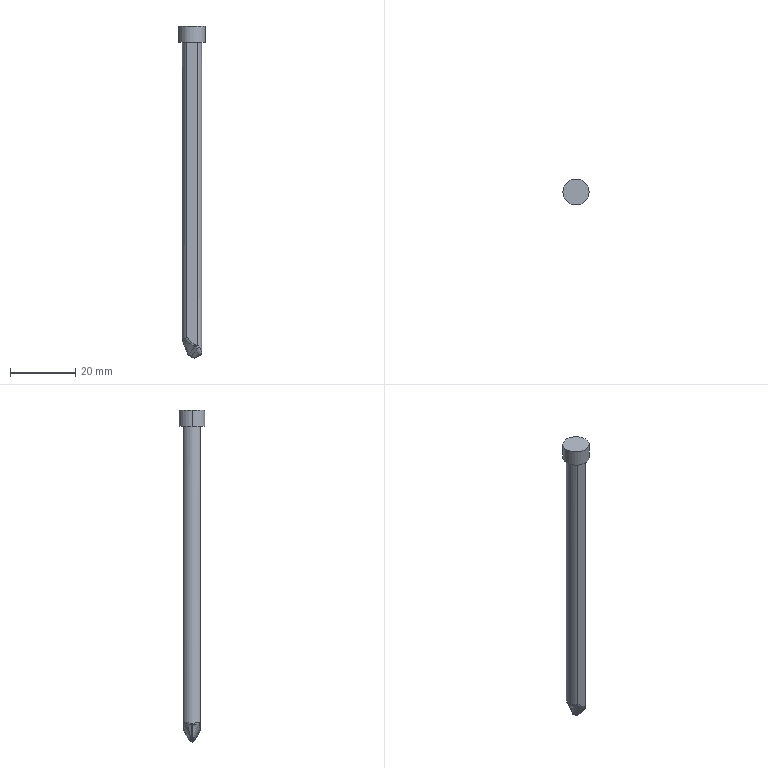Part | 1 solid | 38 faces | box 8 x 8 x 101.756 mm | volume 2706 mm3 | spline 17 | cylinder 8 | plane 7 | torus 4 | other 2 | commonest cylinder face diameters 0.7 x2 2.9 x2 6 x2 8 x2